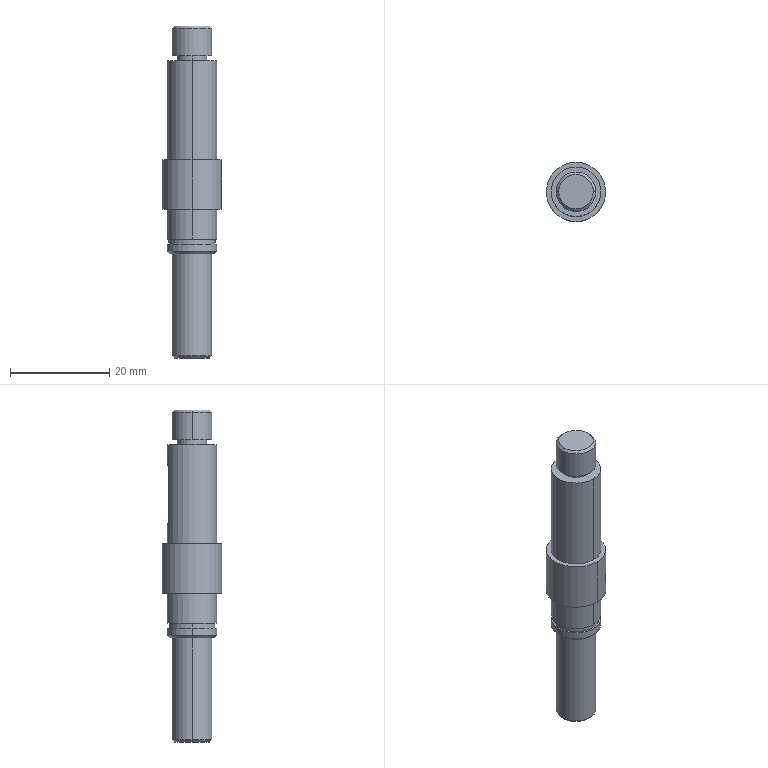Part | STEP file | 06-05 Support feed wheel shaft | 1 solid | 37 faces | box 12 x 12 x 67 mm | volume 4710 mm3 | cylinder 19 | plane 12 | cone 6 | commonest cylinder face diameters 10 x6 8 x4 3 x3 6 x2 9.3 x2 12 x2